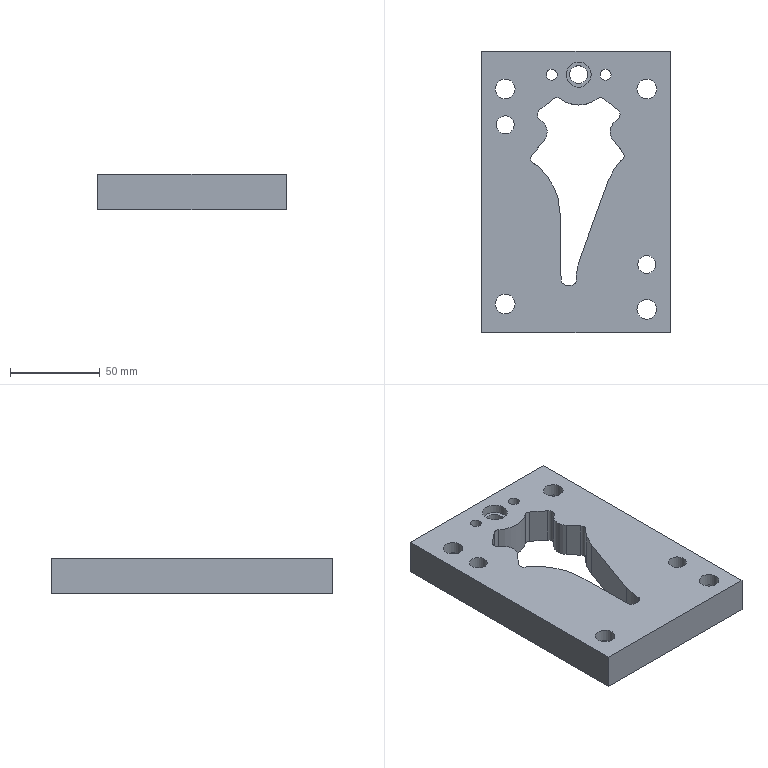Part | STEP file | 408_id3162_x_t | 1 solid | 68 faces | box 105 x 157 x 20 mm | volume 244863 mm3 | cylinder 33 | plane 28 | spline 7 | commonest cylinder face diameters 6 x6 11 x6 14 x5 17 x4 10 x3 4 x2